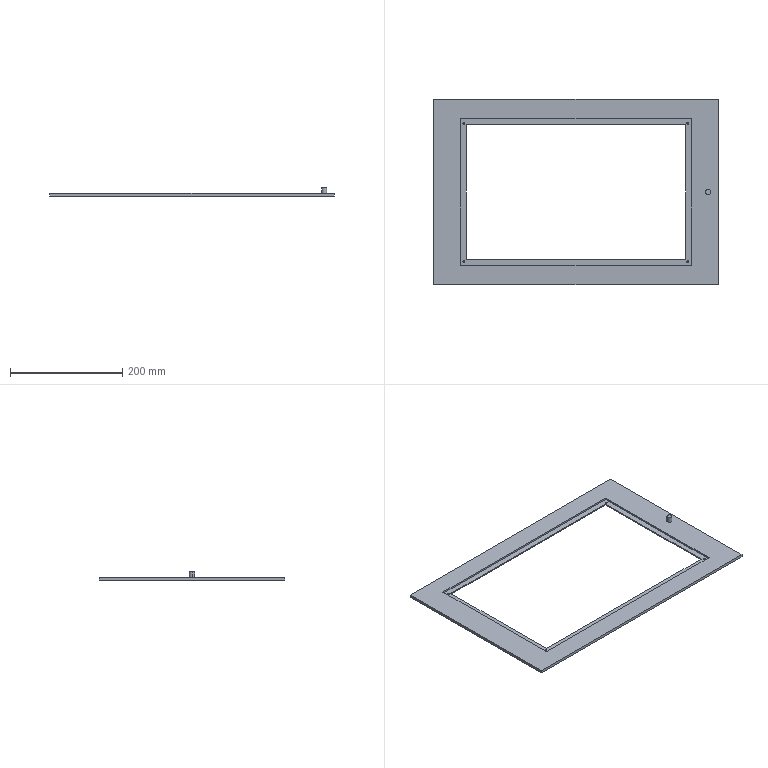Part | STEP file | MYT-A01-P15 | 1 solid | 26 faces | box 506 x 330 x 15 mm | volume 328468 mm3 | plane 16 | cylinder 10 | commonest cylinder face diameters 3.3 x8 9 x2
STEP:
#1=CARTESIAN_POINT('',(239.743,0.,15.));
#2=VERTEX_POINT('',#1);
#3=CARTESIAN_POINT('',(230.743,0.,15.));
#4=VERTEX_POINT('',#3);
#5=CARTESIAN_POINT('',(235.243,0.,15.));
#6=DIRECTION('',(0.,0.,1.));
#7=DIRECTION('',(1.,0.,0.));
#8=AXIS2_PLACEMENT_3D('',#5,#6,#7);
#9=CIRCLE('',#8,4.5);
#10=EDGE_CURVE('',#2,#4,#9,.T.);
#11=ORIENTED_EDGE('',*,*,#10,.F.);
#12=CARTESIAN_POINT('',(239.743,0.,5.));
#13=VERTEX_POINT('',#12);
#14=CARTESIAN_POINT('',(239.743,0.,15.));
#15=DIRECTION('',(0.,0.,-1.));
#16=VECTOR('',#15,1000.);
#17=LINE('',#14,#16);
#18=EDGE_CURVE('',#2,#13,#17,.T.);
#19=ORIENTED_EDGE('',*,*,#18,.T.);
#20=CARTESIAN_POINT('',(230.743,0.,5.));
#21=VERTEX_POINT('',#20);
#22=CARTESIAN_POINT('',(235.243,0.,5.));
#23=DIRECTION('',(0.,0.,1.));
#24=DIRECTION('',(1.,0.,0.));
#25=AXIS2_PLACEMENT_3D('',#22,#23,#24);
#26=CIRCLE('',#25,4.5);
#27=EDGE_CURVE('',#13,#21,#26,.T.);
#28=ORIENTED_EDGE('',*,*,#27,.T.);
#29=CARTESIAN_POINT('',(230.743,0.,15.));
#30=DIRECTION('',(0.,0.,-1.));
#31=VECTOR('',#30,1000.);
#32=LINE('',#29,#31);
#33=EDGE_CURVE('',#4,#21,#32,.T.);
#34=ORIENTED_EDGE('',*,*,#33,.F.);
#35=EDGE_LOOP('',(#11,#19,#28,#34));
#36=FACE_OUTER_BOUND('',#35,.T.);
#37=CARTESIAN_POINT('',(235.243,0.,15.));
#38=DIRECTION('',(0.,0.,-1.));
#39=DIRECTION('',(-1.,0.,0.));
#40=AXIS2_PLACEMENT_3D('',#37,#38,#39);
#41=CYLINDRICAL_SURFACE('',#40,4.5);
#42=ADVANCED_FACE('',(#36),#41,.T.);
#43=CARTESIAN_POINT('',(-201.269,122.337,0.));
#44=VERTEX_POINT('',#43);
#45=CARTESIAN_POINT('',(-197.969,122.337,0.));
#46=VERTEX_POINT('',#45);
#47=CARTESIAN_POINT('',(-199.619,122.337,0.));
#48=DIRECTION('',(0.,0.,1.));
#49=DIRECTION('',(1.,0.,0.));
#50=AXIS2_PLACEMENT_3D('',#47,#48,#49);
#51=CIRCLE('',#50,1.65);
#52=EDGE_CURVE('',#44,#46,#51,.T.);
#53=ORIENTED_EDGE('',*,*,#52,.F.);
#54=CARTESIAN_POINT('',(-201.269,122.337,2.));
#55=VERTEX_POINT('',#54);
#56=CARTESIAN_POINT('',(-201.269,122.337,2.));
#57=DIRECTION('',(0.,0.,1.));
#58=VECTOR('',#57,1000.);
#59=LINE('',#56,#58);
#60=EDGE_CURVE('',#44,#55,#59,.T.);
#61=ORIENTED_EDGE('',*,*,#60,.T.);
#62=CARTESIAN_POINT('',(-197.969,122.337,2.));
#63=VERTEX_POINT('',#62);
#64=CARTESIAN_POINT('',(-199.619,122.337,2.));
#65=DIRECTION('',(0.,0.,1.));
#66=DIRECTION('',(1.,0.,0.));
#67=AXIS2_PLACEMENT_3D('',#64,#65,#66);
#68=CIRCLE('',#67,1.65);
#69=EDGE_CURVE('',#55,#63,#68,.T.);
#70=ORIENTED_EDGE('',*,*,#69,.T.);
#71=CARTESIAN_POINT('',(-197.969,122.337,2.));
#72=DIRECTION('',(0.,0.,1.));
#73=VECTOR('',#72,1000.);
#74=LINE('',#71,#73);
#75=EDGE_CURVE('',#46,#63,#74,.T.);
#76=ORIENTED_EDGE('',*,*,#75,.F.);
#77=EDGE_LOOP('',(#53,#61,#70,#76));
#78=FACE_OUTER_BOUND('',#77,.T.);
#79=CARTESIAN_POINT('',(-199.619,122.337,2.));
#80=DIRECTION('',(0.,0.,1.));
#81=DIRECTION('',(1.,0.,0.));
#82=AXIS2_PLACEMENT_3D('',#79,#80,#81);
#83=CYLINDRICAL_SURFACE('',#82,1.65);
#84=ADVANCED_FACE('',(#78),#83,.F.);
#85=CARTESIAN_POINT('',(-201.269,-124.072,0.));
#86=VERTEX_POINT('',#85);
#87=CARTESIAN_POINT('',(-197.969,-124.072,0.));
#88=VERTEX_POINT('',#87);
#89=CARTESIAN_POINT('',(-199.619,-124.072,0.));
#90=DIRECTION('',(0.,0.,1.));
#91=DIRECTION('',(1.,0.,0.));
#92=AXIS2_PLACEMENT_3D('',#89,#90,#91);
#93=CIRCLE('',#92,1.65);
#94=EDGE_CURVE('',#86,#88,#93,.T.);
#95=ORIENTED_EDGE('',*,*,#94,.F.);
#96=CARTESIAN_POINT('',(-201.269,-124.072,2.));
#97=VERTEX_POINT('',#96);
#98=CARTESIAN_POINT('',(-201.269,-124.072,2.));
#99=DIRECTION('',(0.,0.,1.));
#100=VECTOR('',#99,1000.);
#101=LINE('',#98,#100);
#102=EDGE_CURVE('',#86,#97,#101,.T.);
#103=ORIENTED_EDGE('',*,*,#102,.T.);
#104=CARTESIAN_POINT('',(-197.969,-124.072,2.));
#105=VERTEX_POINT('',#104);
#106=CARTESIAN_POINT('',(-199.619,-124.072,2.));
#107=DIRECTION('',(0.,0.,1.));
#108=DIRECTION('',(1.,0.,0.));
#109=AXIS2_PLACEMENT_3D('',#106,#107,#108);
#110=CIRCLE('',#109,1.65);
#111=EDGE_CURVE('',#97,#105,#110,.T.);
#112=ORIENTED_EDGE('',*,*,#111,.T.);
#113=CARTESIAN_POINT('',(-197.969,-124.072,2.));
#114=DIRECTION('',(0.,0.,1.));
#115=VECTOR('',#114,1000.);
#116=LINE('',#113,#115);
#117=EDGE_CURVE('',#88,#105,#116,.T.);
#118=ORIENTED_EDGE('',*,*,#117,.F.);
#119=EDGE_LOOP('',(#95,#103,#112,#118));
#120=FACE_OUTER_BOUND('',#119,.T.);
#121=CARTESIAN_POINT('',(-199.619,-124.072,2.));
#122=DIRECTION('',(0.,0.,1.));
#123=DIRECTION('',(1.,0.,0.));
#124=AXIS2_PLACEMENT_3D('',#121,#122,#123);
#125=CYLINDRICAL_SURFACE('',#124,1.65);
#126=ADVANCED_FACE('',(#120),#125,.F.);
#127=CARTESIAN_POINT('',(197.313,122.337,0.));
#128=VERTEX_POINT('',#127);
#129=CARTESIAN_POINT('',(200.613,122.337,0.));
#130=VERTEX_POINT('',#129);
#131=CARTESIAN_POINT('',(198.963,122.337,0.));
#132=DIRECTION('',(0.,0.,1.));
#133=DIRECTION('',(1.,0.,0.));
#134=AXIS2_PLACEMENT_3D('',#131,#132,#133);
#135=CIRCLE('',#134,1.65);
#136=EDGE_CURVE('',#128,#130,#135,.T.);
#137=ORIENTED_EDGE('',*,*,#136,.F.);
#138=CARTESIAN_POINT('',(197.313,122.337,2.));
#139=VERTEX_POINT('',#138);
#140=CARTESIAN_POINT('',(197.313,122.337,2.));
#141=DIRECTION('',(0.,0.,1.));
#142=VECTOR('',#141,1000.);
#143=LINE('',#140,#142);
#144=EDGE_CURVE('',#128,#139,#143,.T.);
#145=ORIENTED_EDGE('',*,*,#144,.T.);
#146=CARTESIAN_POINT('',(200.613,122.337,2.));
#147=VERTEX_POINT('',#146);
#148=CARTESIAN_POINT('',(198.963,122.337,2.));
#149=DIRECTION('',(0.,0.,1.));
#150=DIRECTION('',(1.,0.,0.));
#151=AXIS2_PLACEMENT_3D('',#148,#149,#150);
#152=CIRCLE('',#151,1.65);
#153=EDGE_CURVE('',#139,#147,#152,.T.);
#154=ORIENTED_EDGE('',*,*,#153,.T.);
#155=CARTESIAN_POINT('',(200.613,122.337,2.));
#156=DIRECTION('',(0.,0.,1.));
#157=VECTOR('',#156,1000.);
#158=LINE('',#155,#157);
#159=EDGE_CURVE('',#130,#147,#158,.T.);
#160=ORIENTED_EDGE('',*,*,#159,.F.);
#161=EDGE_LOOP('',(#137,#145,#154,#160));
#162=FACE_OUTER_BOUND('',#161,.T.);
#163=CARTESIAN_POINT('',(198.963,122.337,2.));
#164=DIRECTION('',(0.,0.,1.));
#165=DIRECTION('',(1.,0.,0.));
#166=AXIS2_PLACEMENT_3D('',#163,#164,#165);
#167=CYLINDRICAL_SURFACE('',#166,1.65);
#168=ADVANCED_FACE('',(#162),#167,.F.);
#169=CARTESIAN_POINT('',(197.313,-124.072,0.));
#170=VERTEX_POINT('',#169);
#171=CARTESIAN_POINT('',(200.613,-124.072,0.));
#172=VERTEX_POINT('',#171);
#173=CARTESIAN_POINT('',(198.963,-124.072,0.));
#174=DIRECTION('',(0.,0.,1.));
#175=DIRECTION('',(1.,0.,0.));
#176=AXIS2_PLACEMENT_3D('',#173,#174,#175);
#177=CIRCLE('',#176,1.65);
#178=EDGE_CURVE('',#170,#172,#177,.T.);
#179=ORIENTED_EDGE('',*,*,#178,.F.);
#180=CARTESIAN_POINT('',(197.313,-124.072,2.));
#181=VERTEX_POINT('',#180);
#182=CARTESIAN_POINT('',(197.313,-124.072,2.));
#183=DIRECTION('',(0.,0.,1.));
#184=VECTOR('',#183,1000.);
#185=LINE('',#182,#184);
#186=EDGE_CURVE('',#170,#181,#185,.T.);
#187=ORIENTED_EDGE('',*,*,#186,.T.);
#188=CARTESIAN_POINT('',(200.613,-124.072,2.));
#189=VERTEX_POINT('',#188);
#190=CARTESIAN_POINT('',(198.963,-124.072,2.));
#191=DIRECTION('',(0.,0.,1.));
#192=DIRECTION('',(1.,0.,0.));
#193=AXIS2_PLACEMENT_3D('',#190,#191,#192);
#194=CIRCLE('',#193,1.65);
#195=EDGE_CURVE('',#181,#189,#194,.T.);
#196=ORIENTED_EDGE('',*,*,#195,.T.);
#197=CARTESIAN_POINT('',(200.613,-124.072,2.));
#198=DIRECTION('',(0.,0.,1.));
#199=VECTOR('',#198,1000.);
#200=LINE('',#197,#199);
#201=EDGE_CURVE('',#172,#189,#200,.T.);
#202=ORIENTED_EDGE('',*,*,#201,.F.);
#203=EDGE_LOOP('',(#179,#187,#196,#202));
#204=FACE_OUTER_BOUND('',#203,.T.);
#205=CARTESIAN_POINT('',(198.963,-124.072,2.));
#206=DIRECTION('',(0.,0.,1.));
#207=DIRECTION('',(1.,0.,0.));
#208=AXIS2_PLACEMENT_3D('',#205,#206,#207);
#209=CYLINDRICAL_SURFACE('',#208,1.65);
#210=ADVANCED_FACE('',(#204),#209,.F.);
#211=CARTESIAN_POINT('',(195.,120.,2.));
#212=VERTEX_POINT('',#211);
#213=CARTESIAN_POINT('',(195.,-120.,2.));
#214=VERTEX_POINT('',#213);
#215=CARTESIAN_POINT('',(195.,120.,2.));
#216=DIRECTION('',(0.,-1.,0.));
#217=VECTOR('',#216,1000.);
#218=LINE('',#215,#217);
#219=EDGE_CURVE('',#212,#214,#218,.T.);
#220=ORIENTED_EDGE('',*,*,#219,.F.);
#221=CARTESIAN_POINT('',(195.,120.,0.));
#222=VERTEX_POINT('',#221);
#223=CARTESIAN_POINT('',(195.,120.,-5.));
#224=DIRECTION('',(0.,0.,1.));
#225=VECTOR('',#224,1000.);
#226=LINE('',#223,#225);
#227=EDGE_CURVE('',#222,#212,#226,.T.);
#228=ORIENTED_EDGE('',*,*,#227,.F.);
#229=CARTESIAN_POINT('',(195.,-120.,0.));
#230=VERTEX_POINT('',#229);
#231=CARTESIAN_POINT('',(195.,0.,0.));
#232=DIRECTION('',(0.,1.,0.));
#233=VECTOR('',#232,1000.);
#234=LINE('',#231,#233);
#235=EDGE_CURVE('',#230,#222,#234,.T.);
#236=ORIENTED_EDGE('',*,*,#235,.F.);
#237=CARTESIAN_POINT('',(195.,-120.,-5.));
#238=DIRECTION('',(0.,0.,1.));
#239=VECTOR('',#238,1000.);
#240=LINE('',#237,#239);
#241=EDGE_CURVE('',#230,#214,#240,.T.);
#242=ORIENTED_EDGE('',*,*,#241,.T.);
#243=EDGE_LOOP('',(#220,#228,#236,#242));
#244=FACE_OUTER_BOUND('',#243,.T.);
#245=CARTESIAN_POINT('',(195.,120.,-5.));
#246=DIRECTION('',(1.,0.,0.));
#247=DIRECTION('',(0.,1.,0.));
#248=AXIS2_PLACEMENT_3D('',#245,#246,#247);
#249=PLANE('',#248);
#250=ADVANCED_FACE('',(#244),#249,.F.);
#251=CARTESIAN_POINT('',(-195.,-120.,2.));
#252=VERTEX_POINT('',#251);
#253=CARTESIAN_POINT('',(-195.,-120.,2.));
#254=DIRECTION('',(-1.,0.,0.));
#255=VECTOR('',#254,1000.);
#256=LINE('',#253,#255);
#257=EDGE_CURVE('',#214,#252,#256,.T.);
#258=ORIENTED_EDGE('',*,*,#257,.F.);
#259=ORIENTED_EDGE('',*,*,#241,.F.);
#260=CARTESIAN_POINT('',(-195.,-120.,0.));
#261=VERTEX_POINT('',#260);
#262=CARTESIAN_POINT('',(0.,-120.,0.));
#263=DIRECTION('',(1.,0.,0.));
#264=VECTOR('',#263,1000.);
#265=LINE('',#262,#264);
#266=EDGE_CURVE('',#261,#230,#265,.T.);
#267=ORIENTED_EDGE('',*,*,#266,.F.);
#268=CARTESIAN_POINT('',(-195.,-120.,-5.));
#269=DIRECTION('',(0.,0.,1.));
#270=VECTOR('',#269,1000.);
#271=LINE('',#268,#270);
#272=EDGE_CURVE('',#261,#252,#271,.T.);
#273=ORIENTED_EDGE('',*,*,#272,.T.);
#274=EDGE_LOOP('',(#258,#259,#267,#273));
#275=FACE_OUTER_BOUND('',#274,.T.);
#276=CARTESIAN_POINT('',(-195.,-120.,-5.));
#277=DIRECTION('',(0.,-1.,0.));
#278=DIRECTION('',(0.,0.,-1.));
#279=AXIS2_PLACEMENT_3D('',#276,#277,#278);
#280=PLANE('',#279);
#281=ADVANCED_FACE('',(#275),#280,.F.);
#282=CARTESIAN_POINT('',(-195.,120.,2.));
#283=VERTEX_POINT('',#282);
#284=CARTESIAN_POINT('',(-195.,120.,2.));
#285=DIRECTION('',(0.,1.,0.));
#286=VECTOR('',#285,1000.);
#287=LINE('',#284,#286);
#288=EDGE_CURVE('',#252,#283,#287,.T.);
#289=ORIENTED_EDGE('',*,*,#288,.F.);
#290=ORIENTED_EDGE('',*,*,#272,.F.);
#291=CARTESIAN_POINT('',(-195.,120.,0.));
#292=VERTEX_POINT('',#291);
#293=CARTESIAN_POINT('',(-195.,0.,0.));
#294=DIRECTION('',(0.,-1.,0.));
#295=VECTOR('',#294,1000.);
#296=LINE('',#293,#295);
#297=EDGE_CURVE('',#292,#261,#296,.T.);
#298=ORIENTED_EDGE('',*,*,#297,.F.);
#299=CARTESIAN_POINT('',(-195.,120.,-5.));
#300=DIRECTION('',(0.,0.,1.));
#301=VECTOR('',#300,1000.);
#302=LINE('',#299,#301);
#303=EDGE_CURVE('',#292,#283,#302,.T.);
#304=ORIENTED_EDGE('',*,*,#303,.T.);
#305=EDGE_LOOP('',(#289,#290,#298,#304));
#306=FACE_OUTER_BOUND('',#305,.T.);
#307=CARTESIAN_POINT('',(-195.,120.,-5.));
#308=DIRECTION('',(-1.,0.,0.));
#309=DIRECTION('',(0.,-1.,0.));
#310=AXIS2_PLACEMENT_3D('',#307,#308,#309);
#311=PLANE('',#310);
#312=ADVANCED_FACE('',(#306),#311,.F.);
#313=CARTESIAN_POINT('',(-195.,120.,2.));
#314=DIRECTION('',(1.,0.,0.));
#315=VECTOR('',#314,1000.);
#316=LINE('',#313,#315);
#317=EDGE_CURVE('',#283,#212,#316,.T.);
#318=ORIENTED_EDGE('',*,*,#317,.F.);
#319=ORIENTED_EDGE('',*,*,#303,.F.);
#320=CARTESIAN_POINT('',(0.,120.,0.));
#321=DIRECTION('',(-1.,0.,0.));
#322=VECTOR('',#321,1000.);
#323=LINE('',#320,#322);
#324=EDGE_CURVE('',#222,#292,#323,.T.);
#325=ORIENTED_EDGE('',*,*,#324,.F.);
#326=ORIENTED_EDGE('',*,*,#227,.T.);
#327=EDGE_LOOP('',(#318,#319,#325,#326));
#328=FACE_OUTER_BOUND('',#327,.T.);
#329=CARTESIAN_POINT('',(-195.,120.,-5.));
#330=DIRECTION('',(0.,1.,0.));
#331=DIRECTION('',(0.,0.,1.));
#332=AXIS2_PLACEMENT_3D('',#329,#330,#331);
#333=PLANE('',#332);
#334=ADVANCED_FACE('',(#328),#333,.F.);
#335=CARTESIAN_POINT('',(253.,-165.,0.));
#336=VERTEX_POINT('',#335);
#337=CARTESIAN_POINT('',(253.,165.,0.));
#338=VERTEX_POINT('',#337);
#339=CARTESIAN_POINT('',(253.,165.,0.));
#340=DIRECTION('',(0.,1.,0.));
#341=VECTOR('',#340,1000.);
#342=LINE('',#339,#341);
#343=EDGE_CURVE('',#336,#338,#342,.T.);
#344=ORIENTED_EDGE('',*,*,#343,.T.);
#345=CARTESIAN_POINT('',(253.,165.,5.));
#346=VERTEX_POINT('',#345);
#347=CARTESIAN_POINT('',(253.,165.,5.));
#348=DIRECTION('',(0.,0.,-1.));
#349=VECTOR('',#348,1000.);
#350=LINE('',#347,#349);
#351=EDGE_CURVE('',#346,#338,#350,.T.);
#352=ORIENTED_EDGE('',*,*,#351,.F.);
#353=CARTESIAN_POINT('',(253.,-165.,5.));
#354=VERTEX_POINT('',#353);
#355=CARTESIAN_POINT('',(253.,165.,5.));
#356=DIRECTION('',(0.,1.,0.));
#357=VECTOR('',#356,1000.);
#358=LINE('',#355,#357);
#359=EDGE_CURVE('',#354,#346,#358,.T.);
#360=ORIENTED_EDGE('',*,*,#359,.F.);
#361=CARTESIAN_POINT('',(253.,-165.,5.));
#362=DIRECTION('',(0.,0.,-1.));
#363=VECTOR('',#362,1000.);
#364=LINE('',#361,#363);
#365=EDGE_CURVE('',#354,#336,#364,.T.);
#366=ORIENTED_EDGE('',*,*,#365,.T.);
#367=EDGE_LOOP('',(#344,#352,#360,#366));
#368=FACE_OUTER_BOUND('',#367,.T.);
#369=CARTESIAN_POINT('',(253.,165.,5.));
#370=DIRECTION('',(-1.,0.,0.));
#371=DIRECTION('',(0.,-1.,0.));
#372=AXIS2_PLACEMENT_3D('',#369,#370,#371);
#373=PLANE('',#372);
#374=ADVANCED_FACE('',(#368),#373,.F.);
#375=CARTESIAN_POINT('',(-253.,165.,0.));
#376=VERTEX_POINT('',#375);
#377=CARTESIAN_POINT('',(-253.,165.,0.));
#378=DIRECTION('',(-1.,0.,0.));
#379=VECTOR('',#378,1000.);
#380=LINE('',#377,#379);
#381=EDGE_CURVE('',#338,#376,#380,.T.);
#382=ORIENTED_EDGE('',*,*,#381,.T.);
#383=CARTESIAN_POINT('',(-253.,165.,5.));
#384=VERTEX_POINT('',#383);
#385=CARTESIAN_POINT('',(-253.,165.,5.));
#386=DIRECTION('',(0.,0.,-1.));
#387=VECTOR('',#386,1000.);
#388=LINE('',#385,#387);
#389=EDGE_CURVE('',#384,#376,#388,.T.);
#390=ORIENTED_EDGE('',*,*,#389,.F.);
#391=CARTESIAN_POINT('',(-253.,165.,5.));
#392=DIRECTION('',(-1.,0.,0.));
#393=VECTOR('',#392,1000.);
#394=LINE('',#391,#393);
#395=EDGE_CURVE('',#346,#384,#394,.T.);
#396=ORIENTED_EDGE('',*,*,#395,.F.);
#397=ORIENTED_EDGE('',*,*,#351,.T.);
#398=EDGE_LOOP('',(#382,#390,#396,#397));
#399=FACE_OUTER_BOUND('',#398,.T.);
#400=CARTESIAN_POINT('',(-253.,165.,5.));
#401=DIRECTION('',(0.,-1.,0.));
#402=DIRECTION('',(0.,0.,-1.));
#403=AXIS2_PLACEMENT_3D('',#400,#401,#402);
#404=PLANE('',#403);
#405=ADVANCED_FACE('',(#399),#404,.F.);
#406=CARTESIAN_POINT('',(-253.,-165.,0.));
#407=VERTEX_POINT('',#406);
#408=CARTESIAN_POINT('',(-253.,165.,0.));
#409=DIRECTION('',(0.,-1.,0.));
#410=VECTOR('',#409,1000.);
#411=LINE('',#408,#410);
#412=EDGE_CURVE('',#376,#407,#411,.T.);
#413=ORIENTED_EDGE('',*,*,#412,.T.);
#414=CARTESIAN_POINT('',(-253.,-165.,5.));
#415=VERTEX_POINT('',#414);
#416=CARTESIAN_POINT('',(-253.,-165.,5.));
#417=DIRECTION('',(0.,0.,-1.));
#418=VECTOR('',#417,1000.);
#419=LINE('',#416,#418);
#420=EDGE_CURVE('',#415,#407,#419,.T.);
#421=ORIENTED_EDGE('',*,*,#420,.F.);
#422=CARTESIAN_POINT('',(-253.,165.,5.));
#423=DIRECTION('',(0.,-1.,0.));
#424=VECTOR('',#423,1000.);
#425=LINE('',#422,#424);
#426=EDGE_CURVE('',#384,#415,#425,.T.);
#427=ORIENTED_EDGE('',*,*,#426,.F.);
#428=ORIENTED_EDGE('',*,*,#389,.T.);
#429=EDGE_LOOP('',(#413,#421,#427,#428));
#430=FACE_OUTER_BOUND('',#429,.T.);
#431=CARTESIAN_POINT('',(-253.,165.,5.));
#432=DIRECTION('',(1.,0.,0.));
#433=DIRECTION('',(0.,1.,0.));
#434=AXIS2_PLACEMENT_3D('',#431,#432,#433);
#435=PLANE('',#434);
#436=ADVANCED_FACE('',(#430),#435,.F.);
#437=CARTESIAN_POINT('',(-253.,-165.,0.));
#438=DIRECTION('',(1.,0.,0.));
#439=VECTOR('',#438,1000.);
#440=LINE('',#437,#439);
#441=EDGE_CURVE('',#407,#336,#440,.T.);
#442=ORIENTED_EDGE('',*,*,#441,.T.);
#443=ORIENTED_EDGE('',*,*,#365,.F.);
#444=CARTESIAN_POINT('',(-253.,-165.,5.));
#445=DIRECTION('',(1.,0.,0.));
#446=VECTOR('',#445,1000.);
#447=LINE('',#444,#446);
#448=EDGE_CURVE('',#415,#354,#447,.T.);
#449=ORIENTED_EDGE('',*,*,#448,.F.);
#450=ORIENTED_EDGE('',*,*,#420,.T.);
#451=EDGE_LOOP('',(#442,#443,#449,#450));
#452=FACE_OUTER_BOUND('',#451,.T.);
#453=CARTESIAN_POINT('',(-253.,-165.,5.));
#454=DIRECTION('',(0.,1.,0.));
#455=DIRECTION('',(0.,0.,1.));
#456=AXIS2_PLACEMENT_3D('',#453,#454,#455);
#457=PLANE('',#456);
#458=ADVANCED_FACE('',(#452),#457,.F.);
#459=CARTESIAN_POINT('',(235.243,0.,5.));
#460=DIRECTION('',(0.,0.,1.));
#461=DIRECTION('',(1.,0.,0.));
#462=AXIS2_PLACEMENT_3D('',#459,#460,#461);
#463=CIRCLE('',#462,4.5);
#464=EDGE_CURVE('',#21,#13,#463,.T.);
#465=ORIENTED_EDGE('',*,*,#464,.F.);
#466=ORIENTED_EDGE('',*,*,#27,.F.);
#467=EDGE_LOOP('',(#465,#466));
#468=FACE_BOUND('',#467,.T.);
#469=CARTESIAN_POINT('',(205.,-130.,5.));
#470=VERTEX_POINT('',#469);
#471=CARTESIAN_POINT('',(205.,130.,5.));
#472=VERTEX_POINT('',#471);
#473=CARTESIAN_POINT('',(205.,130.,5.));
#474=DIRECTION('',(0.,1.,0.));
#475=VECTOR('',#474,1000.);
#476=LINE('',#473,#475);
#477=EDGE_CURVE('',#470,#472,#476,.T.);
#478=ORIENTED_EDGE('',*,*,#477,.F.);
#479=CARTESIAN_POINT('',(-205.,-130.,5.));
#480=VERTEX_POINT('',#479);
#481=CARTESIAN_POINT('',(-205.,-130.,5.));
#482=DIRECTION('',(1.,0.,0.));
#483=VECTOR('',#482,1000.);
#484=LINE('',#481,#483);
#485=EDGE_CURVE('',#480,#470,#484,.T.);
#486=ORIENTED_EDGE('',*,*,#485,.F.);
#487=CARTESIAN_POINT('',(-205.,130.,5.));
#488=VERTEX_POINT('',#487);
#489=CARTESIAN_POINT('',(-205.,130.,5.));
#490=DIRECTION('',(0.,-1.,0.));
#491=VECTOR('',#490,1000.);
#492=LINE('',#489,#491);
#493=EDGE_CURVE('',#488,#480,#492,.T.);
#494=ORIENTED_EDGE('',*,*,#493,.F.);
#495=CARTESIAN_POINT('',(-205.,130.,5.));
#496=DIRECTION('',(-1.,0.,0.));
#497=VECTOR('',#496,1000.);
#498=LINE('',#495,#497);
#499=EDGE_CURVE('',#472,#488,#498,.T.);
#500=ORIENTED_EDGE('',*,*,#499,.F.);
#501=EDGE_LOOP('',(#478,#486,#494,#500));
#502=FACE_BOUND('',#501,.T.);
#503=ORIENTED_EDGE('',*,*,#359,.T.);
#504=ORIENTED_EDGE('',*,*,#395,.T.);
#505=ORIENTED_EDGE('',*,*,#426,.T.);
#506=ORIENTED_EDGE('',*,*,#448,.T.);
#507=EDGE_LOOP('',(#503,#504,#505,#506));
#508=FACE_OUTER_BOUND('',#507,.T.);
#509=CARTESIAN_POINT('',(0.,0.,5.));
#510=DIRECTION('',(0.,0.,1.));
#511=DIRECTION('',(1.,0.,0.));
#512=AXIS2_PLACEMENT_3D('',#509,#510,#511);
#513=PLANE('',#512);
#514=ADVANCED_FACE('',(#468,#502,#508),#513,.T.);
#515=CARTESIAN_POINT('',(-199.619,122.337,0.));
#516=DIRECTION('',(0.,0.,1.));
#517=DIRECTION('',(1.,0.,0.));
#518=AXIS2_PLACEMENT_3D('',#515,#516,#517);
#519=CIRCLE('',#518,1.65);
#520=EDGE_CURVE('',#46,#44,#519,.T.);
#521=ORIENTED_EDGE('',*,*,#520,.T.);
#522=ORIENTED_EDGE('',*,*,#52,.T.);
#523=EDGE_LOOP('',(#521,#522));
#524=FACE_BOUND('',#523,.T.);
#525=CARTESIAN_POINT('',(-199.619,-124.072,0.));
#526=DIRECTION('',(0.,0.,1.));
#527=DIRECTION('',(1.,0.,0.));
#528=AXIS2_PLACEMENT_3D('',#525,#526,#527);
#529=CIRCLE('',#528,1.65);
#530=EDGE_CURVE('',#88,#86,#529,.T.);
#531=ORIENTED_EDGE('',*,*,#530,.T.);
#532=ORIENTED_EDGE('',*,*,#94,.T.);
#533=EDGE_LOOP('',(#531,#532));
#534=FACE_BOUND('',#533,.T.);
#535=CARTESIAN_POINT('',(198.963,122.337,0.));
#536=DIRECTION('',(0.,0.,1.));
#537=DIRECTION('',(1.,0.,0.));
#538=AXIS2_PLACEMENT_3D('',#535,#536,#537);
#539=CIRCLE('',#538,1.65);
#540=EDGE_CURVE('',#130,#128,#539,.T.);
#541=ORIENTED_EDGE('',*,*,#540,.T.);
#542=ORIENTED_EDGE('',*,*,#136,.T.);
#543=EDGE_LOOP('',(#541,#542));
#544=FACE_BOUND('',#543,.T.);
#545=CARTESIAN_POINT('',(198.963,-124.072,0.));
#546=DIRECTION('',(0.,0.,1.));
#547=DIRECTION('',(1.,0.,0.));
#548=AXIS2_PLACEMENT_3D('',#545,#546,#547);
#549=CIRCLE('',#548,1.65);
#550=EDGE_CURVE('',#172,#170,#549,.T.);
#551=ORIENTED_EDGE('',*,*,#550,.T.);
#552=ORIENTED_EDGE('',*,*,#178,.T.);
#553=EDGE_LOOP('',(#551,#552));
#554=FACE_BOUND('',#553,.T.);
#555=ORIENTED_EDGE('',*,*,#266,.T.);
#556=ORIENTED_EDGE('',*,*,#235,.T.);
#557=ORIENTED_EDGE('',*,*,#324,.T.);
#558=ORIENTED_EDGE('',*,*,#297,.T.);
#559=EDGE_LOOP('',(#555,#556,#557,#558));
#560=FACE_BOUND('',#559,.T.);
#561=ORIENTED_EDGE('',*,*,#343,.F.);
#562=ORIENTED_EDGE('',*,*,#441,.F.);
#563=ORIENTED_EDGE('',*,*,#412,.F.);
#564=ORIENTED_EDGE('',*,*,#381,.F.);
#565=EDGE_LOOP('',(#561,#562,#563,#564));
#566=FACE_OUTER_BOUND('',#565,.T.);
#567=CARTESIAN_POINT('',(0.,0.,0.));
#568=DIRECTION('',(0.,0.,1.));
#569=DIRECTION('',(1.,0.,0.));
#570=AXIS2_PLACEMENT_3D('',#567,#568,#569);
#571=PLANE('',#570);
#572=ADVANCED_FACE('',(#524,#534,#544,#554,#560,#566),#571,.F.);
#573=CARTESIAN_POINT('',(-199.619,122.337,2.));
#574=DIRECTION('',(0.,0.,1.));
#575=DIRECTION('',(1.,0.,0.));
#576=AXIS2_PLACEMENT_3D('',#573,#574,#575);
#577=CIRCLE('',#576,1.65);
#578=EDGE_CURVE('',#63,#55,#577,.T.);
#579=ORIENTED_EDGE('',*,*,#578,.F.);
#580=ORIENTED_EDGE('',*,*,#69,.F.);
#581=EDGE_LOOP('',(#579,#580));
#582=FACE_BOUND('',#581,.T.);
#583=CARTESIAN_POINT('',(-199.619,-124.072,2.));
#584=DIRECTION('',(0.,0.,1.));
#585=DIRECTION('',(1.,0.,0.));
#586=AXIS2_PLACEMENT_3D('',#583,#584,#585);
#587=CIRCLE('',#586,1.65);
#588=EDGE_CURVE('',#105,#97,#587,.T.);
#589=ORIENTED_EDGE('',*,*,#588,.F.);
#590=ORIENTED_EDGE('',*,*,#111,.F.);
#591=EDGE_LOOP('',(#589,#590));
#592=FACE_BOUND('',#591,.T.);
#593=CARTESIAN_POINT('',(198.963,122.337,2.));
#594=DIRECTION('',(0.,0.,1.));
#595=DIRECTION('',(1.,0.,0.));
#596=AXIS2_PLACEMENT_3D('',#593,#594,#595);
#597=CIRCLE('',#596,1.65);
#598=EDGE_CURVE('',#147,#139,#597,.T.);
#599=ORIENTED_EDGE('',*,*,#598,.F.);
#600=ORIENTED_EDGE('',*,*,#153,.F.);
#601=EDGE_LOOP('',(#599,#600));
#602=FACE_BOUND('',#601,.T.);
#603=CARTESIAN_POINT('',(198.963,-124.072,2.));
#604=DIRECTION('',(0.,0.,1.));
#605=DIRECTION('',(1.,0.,0.));
#606=AXIS2_PLACEMENT_3D('',#603,#604,#605);
#607=CIRCLE('',#606,1.65);
#608=EDGE_CURVE('',#189,#181,#607,.T.);
#609=ORIENTED_EDGE('',*,*,#608,.F.);
#610=ORIENTED_EDGE('',*,*,#195,.F.);
#611=EDGE_LOOP('',(#609,#610));
#612=FACE_BOUND('',#611,.T.);
#613=CARTESIAN_POINT('',(205.,-130.,2.));
#614=VERTEX_POINT('',#613);
#615=CARTESIAN_POINT('',(205.,130.,2.));
#616=VERTEX_POINT('',#615);
#617=CARTESIAN_POINT('',(205.,130.,2.));
#618=DIRECTION('',(0.,1.,0.));
#619=VECTOR('',#618,1000.);
#620=LINE('',#617,#619);
#621=EDGE_CURVE('',#614,#616,#620,.T.);
#622=ORIENTED_EDGE('',*,*,#621,.T.);
#623=CARTESIAN_POINT('',(-205.,130.,2.));
#624=VERTEX_POINT('',#623);
#625=CARTESIAN_POINT('',(-205.,130.,2.));
#626=DIRECTION('',(-1.,0.,0.));
#627=VECTOR('',#626,1000.);
#628=LINE('',#625,#627);
#629=EDGE_CURVE('',#616,#624,#628,.T.);
#630=ORIENTED_EDGE('',*,*,#629,.T.);
#631=CARTESIAN_POINT('',(-205.,-130.,2.));
#632=VERTEX_POINT('',#631);
#633=CARTESIAN_POINT('',(-205.,130.,2.));
#634=DIRECTION('',(0.,-1.,0.));
#635=VECTOR('',#634,1000.);
#636=LINE('',#633,#635);
#637=EDGE_CURVE('',#624,#632,#636,.T.);
#638=ORIENTED_EDGE('',*,*,#637,.T.);
#639=CARTESIAN_POINT('',(-205.,-130.,2.));
#640=DIRECTION('',(1.,0.,0.));
#641=VECTOR('',#640,1000.);
#642=LINE('',#639,#641);
#643=EDGE_CURVE('',#632,#614,#642,.T.);
#644=ORIENTED_EDGE('',*,*,#643,.T.);
#645=EDGE_LOOP('',(#622,#630,#638,#644));
#646=FACE_OUTER_BOUND('',#645,.T.);
#647=ORIENTED_EDGE('',*,*,#219,.T.);
#648=ORIENTED_EDGE('',*,*,#257,.T.);
#649=ORIENTED_EDGE('',*,*,#288,.T.);
#650=ORIENTED_EDGE('',*,*,#317,.T.);
#651=EDGE_LOOP('',(#647,#648,#649,#650));
#652=FACE_BOUND('',#651,.T.);
#653=CARTESIAN_POINT('',(0.,0.,2.));
#654=DIRECTION('',(0.,0.,1.));
#655=DIRECTION('',(1.,0.,0.));
#656=AXIS2_PLACEMENT_3D('',#653,#654,#655);
#657=PLANE('',#656);
#658=ADVANCED_FACE('',(#582,#592,#602,#612,#646,#652),#657,.T.);
#659=ORIENTED_EDGE('',*,*,#477,.T.);
#660=CARTESIAN_POINT('',(205.,130.,2.));
#661=DIRECTION('',(0.,0.,1.));
#662=VECTOR('',#661,1000.);
#663=LINE('',#660,#662);
#664=EDGE_CURVE('',#616,#472,#663,.T.);
#665=ORIENTED_EDGE('',*,*,#664,.F.);
#666=ORIENTED_EDGE('',*,*,#621,.F.);
#667=CARTESIAN_POINT('',(205.,-130.,2.));
#668=DIRECTION('',(0.,0.,1.));
#669=VECTOR('',#668,1000.);
#670=LINE('',#667,#669);
#671=EDGE_CURVE('',#614,#470,#670,.T.);
#672=ORIENTED_EDGE('',*,*,#671,.T.);
#673=EDGE_LOOP('',(#659,#665,#666,#672));
#674=FACE_OUTER_BOUND('',#673,.T.);
#675=CARTESIAN_POINT('',(205.,130.,2.));
#676=DIRECTION('',(1.,0.,0.));
#677=DIRECTION('',(0.,1.,0.));
#678=AXIS2_PLACEMENT_3D('',#675,#676,#677);
#679=PLANE('',#678);
#680=ADVANCED_FACE('',(#674),#679,.F.);
#681=ORIENTED_EDGE('',*,*,#485,.T.);
#682=ORIENTED_EDGE('',*,*,#671,.F.);
#683=ORIENTED_EDGE('',*,*,#643,.F.);
#684=CARTESIAN_POINT('',(-205.,-130.,2.));
#685=DIRECTION('',(0.,0.,1.));
#686=VECTOR('',#685,1000.);
#687=LINE('',#684,#686);
#688=EDGE_CURVE('',#632,#480,#687,.T.);
#689=ORIENTED_EDGE('',*,*,#688,.T.);
#690=EDGE_LOOP('',(#681,#682,#683,#689));
#691=FACE_OUTER_BOUND('',#690,.T.);
#692=CARTESIAN_POINT('',(-205.,-130.,2.));
#693=DIRECTION('',(0.,-1.,0.));
#694=DIRECTION('',(0.,0.,-1.));
#695=AXIS2_PLACEMENT_3D('',#692,#693,#694);
#696=PLANE('',#695);
#697=ADVANCED_FACE('',(#691),#696,.F.);
#698=ORIENTED_EDGE('',*,*,#493,.T.);
#699=ORIENTED_EDGE('',*,*,#688,.F.);
#700=ORIENTED_EDGE('',*,*,#637,.F.);
#701=CARTESIAN_POINT('',(-205.,130.,2.));
#702=DIRECTION('',(0.,0.,1.));
#703=VECTOR('',#702,1000.);
#704=LINE('',#701,#703);
#705=EDGE_CURVE('',#624,#488,#704,.T.);
#706=ORIENTED_EDGE('',*,*,#705,.T.);
#707=EDGE_LOOP('',(#698,#699,#700,#706));
#708=FACE_OUTER_BOUND('',#707,.T.);
#709=CARTESIAN_POINT('',(-205.,130.,2.));
#710=DIRECTION('',(-1.,0.,0.));
#711=DIRECTION('',(0.,-1.,0.));
#712=AXIS2_PLACEMENT_3D('',#709,#710,#711);
#713=PLANE('',#712);
#714=ADVANCED_FACE('',(#708),#713,.F.);
#715=ORIENTED_EDGE('',*,*,#499,.T.);
#716=ORIENTED_EDGE('',*,*,#705,.F.);
#717=ORIENTED_EDGE('',*,*,#629,.F.);
#718=ORIENTED_EDGE('',*,*,#664,.T.);
#719=EDGE_LOOP('',(#715,#716,#717,#718));
#720=FACE_OUTER_BOUND('',#719,.T.);
#721=CARTESIAN_POINT('',(-205.,130.,2.));
#722=DIRECTION('',(0.,1.,0.));
#723=DIRECTION('',(0.,0.,1.));
#724=AXIS2_PLACEMENT_3D('',#721,#722,#723);
#725=PLANE('',#724);
#726=ADVANCED_FACE('',(#720),#725,.F.);
#727=ORIENTED_EDGE('',*,*,#186,.F.);
#728=ORIENTED_EDGE('',*,*,#550,.F.);
#729=ORIENTED_EDGE('',*,*,#201,.T.);
#730=ORIENTED_EDGE('',*,*,#608,.T.);
#731=EDGE_LOOP('',(#727,#728,#729,#730));
#732=FACE_OUTER_BOUND('',#731,.T.);
#733=CARTESIAN_POINT('',(198.963,-124.072,2.));
#734=DIRECTION('',(0.,0.,1.));
#735=DIRECTION('',(1.,0.,0.));
#736=AXIS2_PLACEMENT_3D('',#733,#734,#735);
#737=CYLINDRICAL_SURFACE('',#736,1.65);
#738=ADVANCED_FACE('',(#732),#737,.F.);
#739=ORIENTED_EDGE('',*,*,#144,.F.);
#740=ORIENTED_EDGE('',*,*,#540,.F.);
#741=ORIENTED_EDGE('',*,*,#159,.T.);
#742=ORIENTED_EDGE('',*,*,#598,.T.);
#743=EDGE_LOOP('',(#739,#740,#741,#742));
#744=FACE_OUTER_BOUND('',#743,.T.);
#745=CARTESIAN_POINT('',(198.963,122.337,2.));
#746=DIRECTION('',(0.,0.,1.));
#747=DIRECTION('',(1.,0.,0.));
#748=AXIS2_PLACEMENT_3D('',#745,#746,#747);
#749=CYLINDRICAL_SURFACE('',#748,1.65);
#750=ADVANCED_FACE('',(#744),#749,.F.);
#751=ORIENTED_EDGE('',*,*,#102,.F.);
#752=ORIENTED_EDGE('',*,*,#530,.F.);
#753=ORIENTED_EDGE('',*,*,#117,.T.);
#754=ORIENTED_EDGE('',*,*,#588,.T.);
#755=EDGE_LOOP('',(#751,#752,#753,#754));
#756=FACE_OUTER_BOUND('',#755,.T.);
#757=CARTESIAN_POINT('',(-199.619,-124.072,2.));
#758=DIRECTION('',(0.,0.,1.));
#759=DIRECTION('',(1.,0.,0.));
#760=AXIS2_PLACEMENT_3D('',#757,#758,#759);
#761=CYLINDRICAL_SURFACE('',#760,1.65);
#762=ADVANCED_FACE('',(#756),#761,.F.);
#763=ORIENTED_EDGE('',*,*,#60,.F.);
#764=ORIENTED_EDGE('',*,*,#520,.F.);
#765=ORIENTED_EDGE('',*,*,#75,.T.);
#766=ORIENTED_EDGE('',*,*,#578,.T.);
#767=EDGE_LOOP('',(#763,#764,#765,#766));
#768=FACE_OUTER_BOUND('',#767,.T.);
#769=CARTESIAN_POINT('',(-199.619,122.337,2.));
#770=DIRECTION('',(0.,0.,1.));
#771=DIRECTION('',(1.,0.,0.));
#772=AXIS2_PLACEMENT_3D('',#769,#770,#771);
#773=CYLINDRICAL_SURFACE('',#772,1.65);
#774=ADVANCED_FACE('',(#768),#773,.F.);
#775=ORIENTED_EDGE('',*,*,#18,.F.);
#776=CARTESIAN_POINT('',(235.243,0.,15.));
#777=DIRECTION('',(0.,0.,1.));
#778=DIRECTION('',(1.,0.,0.));
#779=AXIS2_PLACEMENT_3D('',#776,#777,#778);
#780=CIRCLE('',#779,4.5);
#781=EDGE_CURVE('',#4,#2,#780,.T.);
#782=ORIENTED_EDGE('',*,*,#781,.F.);
#783=ORIENTED_EDGE('',*,*,#33,.T.);
#784=ORIENTED_EDGE('',*,*,#464,.T.);
#785=EDGE_LOOP('',(#775,#782,#783,#784));
#786=FACE_OUTER_BOUND('',#785,.T.);
#787=CARTESIAN_POINT('',(235.243,0.,15.));
#788=DIRECTION('',(0.,0.,-1.));
#789=DIRECTION('',(-1.,0.,0.));
#790=AXIS2_PLACEMENT_3D('',#787,#788,#789);
#791=CYLINDRICAL_SURFACE('',#790,4.5);
#792=ADVANCED_FACE('',(#786),#791,.T.);
#793=ORIENTED_EDGE('',*,*,#781,.T.);
#794=ORIENTED_EDGE('',*,*,#10,.T.);
#795=EDGE_LOOP('',(#793,#794));
#796=FACE_OUTER_BOUND('',#795,.T.);
#797=CARTESIAN_POINT('',(235.243,0.,15.));
#798=DIRECTION('',(0.,0.,1.));
#799=DIRECTION('',(1.,0.,0.));
#800=AXIS2_PLACEMENT_3D('',#797,#798,#799);
#801=PLANE('',#800);
#802=ADVANCED_FACE('',(#796),#801,.T.);
#803=CLOSED_SHELL('',(#42,#84,#126,#168,#210,#250,#281,#312,#334,#374,#405,#436,#458,#514,#572,#658,#680,#697,#714,#726,#738,#750,#762,#774,#792,#802));
#804=MANIFOLD_SOLID_BREP('',#803);
#805=CARTESIAN_POINT('',(0.,0.,0.));
#806=DIRECTION('',(0.,0.,1.));
#807=DIRECTION('',(1.,0.,0.));
#808=AXIS2_PLACEMENT_3D('',#805,#806,#807);
#809=(LENGTH_UNIT()NAMED_UNIT(*)SI_UNIT(.MILLI.,.METRE.));
#810=UNCERTAINTY_MEASURE_WITH_UNIT(LENGTH_MEASURE(0.00001),#809,'','');
#811=(NAMED_UNIT(*)PLANE_ANGLE_UNIT()SI_UNIT($,.RADIAN.));
#812=(NAMED_UNIT(*)SI_UNIT($,.STERADIAN.)SOLID_ANGLE_UNIT());
#813=(GEOMETRIC_REPRESENTATION_CONTEXT(3)GLOBAL_UNCERTAINTY_ASSIGNED_CONTEXT((#810))GLOBAL_UNIT_ASSIGNED_CONTEXT((#809,#811,#812))REPRESENTATION_CONTEXT('',''));
#814=ADVANCED_BREP_SHAPE_REPRESENTATION('',(#804,#808),#813);